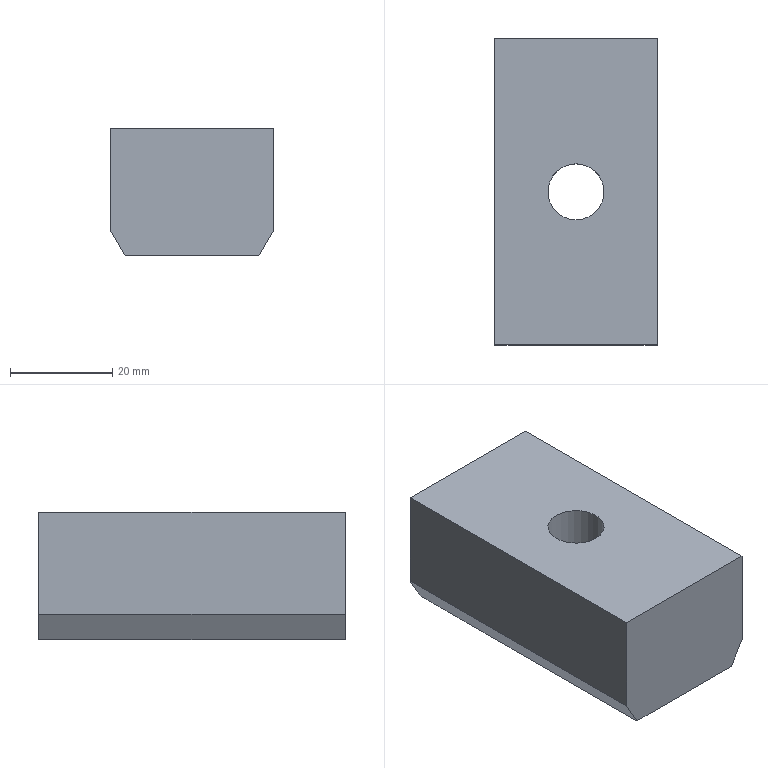Part | NX | features MAIN_BODY 2 | 1 solid | 11 faces | box 32 x 60 x 25 mm | volume 42845 mm3 | plane 9 | cylinder 2 | commonest cylinder face diameters 11 x1 18 x1
STEP:
#1=CARTESIAN_POINT('',(-127.887,-123.5,-120.));
#2=VERTEX_POINT('',#1);
#3=CARTESIAN_POINT('',(-154.113,-123.5,-120.));
#4=VERTEX_POINT('',#3);
#5=CARTESIAN_POINT('',(-125.,-123.5,-120.));
#6=DIRECTION('',(-1.,0.,0.));
#7=VECTOR('',#6,1000.);
#8=LINE('',#5,#7);
#9=EDGE_CURVE('',#2,#4,#8,.T.);
#10=ORIENTED_EDGE('',*,*,#9,.F.);
#11=CARTESIAN_POINT('',(-125.,-123.5,-115.));
#12=VERTEX_POINT('',#11);
#13=CARTESIAN_POINT('',(-127.165,-123.5,-118.75));
#14=DIRECTION('',(-0.5,0.,-0.866));
#15=VECTOR('',#14,1000.);
#16=LINE('',#13,#15);
#17=EDGE_CURVE('',#12,#2,#16,.T.);
#18=ORIENTED_EDGE('',*,*,#17,.F.);
#19=CARTESIAN_POINT('',(-125.,-123.5,-95.));
#20=VERTEX_POINT('',#19);
#21=CARTESIAN_POINT('',(-125.,-123.5,-120.));
#22=DIRECTION('',(0.,0.,1.));
#23=VECTOR('',#22,1000.);
#24=LINE('',#21,#23);
#25=EDGE_CURVE('',#12,#20,#24,.T.);
#26=ORIENTED_EDGE('',*,*,#25,.T.);
#27=CARTESIAN_POINT('',(-157.,-123.5,-95.));
#28=VERTEX_POINT('',#27);
#29=CARTESIAN_POINT('',(-125.,-123.5,-95.));
#30=DIRECTION('',(-1.,0.,0.));
#31=VECTOR('',#30,1000.);
#32=LINE('',#29,#31);
#33=EDGE_CURVE('',#20,#28,#32,.T.);
#34=ORIENTED_EDGE('',*,*,#33,.T.);
#35=CARTESIAN_POINT('',(-157.,-123.5,-115.));
#36=VERTEX_POINT('',#35);
#37=CARTESIAN_POINT('',(-157.,-123.5,-120.));
#38=DIRECTION('',(0.,0.,1.));
#39=VECTOR('',#38,1000.);
#40=LINE('',#37,#39);
#41=EDGE_CURVE('',#36,#28,#40,.T.);
#42=ORIENTED_EDGE('',*,*,#41,.F.);
#43=CARTESIAN_POINT('',(-146.835,-123.5,-132.606));
#44=DIRECTION('',(-0.5,0.,0.866));
#45=VECTOR('',#44,1000.);
#46=LINE('',#43,#45);
#47=EDGE_CURVE('',#4,#36,#46,.T.);
#48=ORIENTED_EDGE('',*,*,#47,.F.);
#49=EDGE_LOOP('',(#10,#18,#26,#34,#42,#48));
#50=FACE_BOUND('',#49,.T.);
#51=CARTESIAN_POINT('',(-125.,-123.5,-120.));
#52=DIRECTION('',(0.,-1.,0.));
#53=DIRECTION('',(1.,0.,0.));
#54=AXIS2_PLACEMENT_3D('',#51,#52,#53);
#55=PLANE('',#54);
#56=ADVANCED_FACE('',(#50),#55,.T.);
#57=ORIENTED_EDGE('',*,*,#41,.T.);
#58=CARTESIAN_POINT('',(-157.,-63.5,-95.));
#59=VERTEX_POINT('',#58);
#60=CARTESIAN_POINT('',(-157.,-123.5,-95.));
#61=DIRECTION('',(0.,1.,0.));
#62=VECTOR('',#61,1000.);
#63=LINE('',#60,#62);
#64=EDGE_CURVE('',#28,#59,#63,.T.);
#65=ORIENTED_EDGE('',*,*,#64,.T.);
#66=CARTESIAN_POINT('',(-157.,-63.5,-115.));
#67=VERTEX_POINT('',#66);
#68=CARTESIAN_POINT('',(-157.,-63.5,-120.));
#69=DIRECTION('',(0.,0.,1.));
#70=VECTOR('',#69,1000.);
#71=LINE('',#68,#70);
#72=EDGE_CURVE('',#67,#59,#71,.T.);
#73=ORIENTED_EDGE('',*,*,#72,.F.);
#74=CARTESIAN_POINT('',(-157.,-63.5,-115.));
#75=DIRECTION('',(0.,1.,0.));
#76=VECTOR('',#75,1000.);
#77=LINE('',#74,#76);
#78=EDGE_CURVE('',#36,#67,#77,.T.);
#79=ORIENTED_EDGE('',*,*,#78,.F.);
#80=EDGE_LOOP('',(#57,#65,#73,#79));
#81=FACE_BOUND('',#80,.T.);
#82=CARTESIAN_POINT('',(-157.,-123.5,-120.));
#83=DIRECTION('',(-1.,0.,0.));
#84=DIRECTION('',(0.,-1.,0.));
#85=AXIS2_PLACEMENT_3D('',#82,#83,#84);
#86=PLANE('',#85);
#87=ADVANCED_FACE('',(#81),#86,.T.);
#88=ORIENTED_EDGE('',*,*,#72,.T.);
#89=CARTESIAN_POINT('',(-125.,-63.5,-95.));
#90=VERTEX_POINT('',#89);
#91=CARTESIAN_POINT('',(-157.,-63.5,-95.));
#92=DIRECTION('',(1.,0.,0.));
#93=VECTOR('',#92,1000.);
#94=LINE('',#91,#93);
#95=EDGE_CURVE('',#59,#90,#94,.T.);
#96=ORIENTED_EDGE('',*,*,#95,.T.);
#97=CARTESIAN_POINT('',(-125.,-63.5,-115.));
#98=VERTEX_POINT('',#97);
#99=CARTESIAN_POINT('',(-125.,-63.5,-120.));
#100=DIRECTION('',(0.,0.,1.));
#101=VECTOR('',#100,1000.);
#102=LINE('',#99,#101);
#103=EDGE_CURVE('',#98,#90,#102,.T.);
#104=ORIENTED_EDGE('',*,*,#103,.F.);
#105=CARTESIAN_POINT('',(-127.887,-63.5,-120.));
#106=VERTEX_POINT('',#105);
#107=CARTESIAN_POINT('',(-135.165,-63.5,-132.606));
#108=DIRECTION('',(0.5,0.,0.866));
#109=VECTOR('',#108,1000.);
#110=LINE('',#107,#109);
#111=EDGE_CURVE('',#106,#98,#110,.T.);
#112=ORIENTED_EDGE('',*,*,#111,.F.);
#113=CARTESIAN_POINT('',(-154.113,-63.5,-120.));
#114=VERTEX_POINT('',#113);
#115=CARTESIAN_POINT('',(-157.,-63.5,-120.));
#116=DIRECTION('',(1.,0.,0.));
#117=VECTOR('',#116,1000.);
#118=LINE('',#115,#117);
#119=EDGE_CURVE('',#114,#106,#118,.T.);
#120=ORIENTED_EDGE('',*,*,#119,.F.);
#121=CARTESIAN_POINT('',(-154.835,-63.5,-118.75));
#122=DIRECTION('',(0.5,0.,-0.866));
#123=VECTOR('',#122,1000.);
#124=LINE('',#121,#123);
#125=EDGE_CURVE('',#67,#114,#124,.T.);
#126=ORIENTED_EDGE('',*,*,#125,.F.);
#127=EDGE_LOOP('',(#88,#96,#104,#112,#120,#126));
#128=FACE_BOUND('',#127,.T.);
#129=CARTESIAN_POINT('',(-157.,-63.5,-120.));
#130=DIRECTION('',(0.,1.,0.));
#131=DIRECTION('',(-1.,0.,0.));
#132=AXIS2_PLACEMENT_3D('',#129,#130,#131);
#133=PLANE('',#132);
#134=ADVANCED_FACE('',(#128),#133,.T.);
#135=ORIENTED_EDGE('',*,*,#103,.T.);
#136=CARTESIAN_POINT('',(-125.,-63.5,-95.));
#137=DIRECTION('',(0.,-1.,0.));
#138=VECTOR('',#137,1000.);
#139=LINE('',#136,#138);
#140=EDGE_CURVE('',#90,#20,#139,.T.);
#141=ORIENTED_EDGE('',*,*,#140,.T.);
#142=ORIENTED_EDGE('',*,*,#25,.F.);
#143=CARTESIAN_POINT('',(-125.,-123.5,-115.));
#144=DIRECTION('',(0.,-1.,0.));
#145=VECTOR('',#144,1000.);
#146=LINE('',#143,#145);
#147=EDGE_CURVE('',#98,#12,#146,.T.);
#148=ORIENTED_EDGE('',*,*,#147,.F.);
#149=EDGE_LOOP('',(#135,#141,#142,#148));
#150=FACE_BOUND('',#149,.T.);
#151=CARTESIAN_POINT('',(-125.,-63.5,-120.));
#152=DIRECTION('',(1.,0.,0.));
#153=DIRECTION('',(0.,0.,-1.));
#154=AXIS2_PLACEMENT_3D('',#151,#152,#153);
#155=PLANE('',#154);
#156=ADVANCED_FACE('',(#150),#155,.T.);
#157=CARTESIAN_POINT('',(-141.,-84.5,-120.));
#158=VERTEX_POINT('',#157);
#159=CARTESIAN_POINT('',(-141.,-93.5,-120.));
#160=DIRECTION('',(0.,0.,-1.));
#161=DIRECTION('',(0.,1.,0.));
#162=AXIS2_PLACEMENT_3D('',#159,#160,#161);
#163=CIRCLE('',#162,9.);
#164=EDGE_CURVE('',#158,#158,#163,.T.);
#165=ORIENTED_EDGE('',*,*,#164,.F.);
#166=EDGE_LOOP('',(#165));
#167=FACE_BOUND('',#166,.T.);
#168=ORIENTED_EDGE('',*,*,#119,.T.);
#169=CARTESIAN_POINT('',(-127.887,-63.5,-120.));
#170=DIRECTION('',(0.,1.,0.));
#171=VECTOR('',#170,1000.);
#172=LINE('',#169,#171);
#173=EDGE_CURVE('',#2,#106,#172,.T.);
#174=ORIENTED_EDGE('',*,*,#173,.F.);
#175=ORIENTED_EDGE('',*,*,#9,.T.);
#176=CARTESIAN_POINT('',(-154.113,-123.5,-120.));
#177=DIRECTION('',(0.,-1.,0.));
#178=VECTOR('',#177,1000.);
#179=LINE('',#176,#178);
#180=EDGE_CURVE('',#114,#4,#179,.T.);
#181=ORIENTED_EDGE('',*,*,#180,.F.);
#182=EDGE_LOOP('',(#168,#174,#175,#181));
#183=FACE_BOUND('',#182,.T.);
#184=CARTESIAN_POINT('',(-157.,-123.5,-120.));
#185=DIRECTION('',(0.,0.,1.));
#186=DIRECTION('',(0.,1.,0.));
#187=AXIS2_PLACEMENT_3D('',#184,#185,#186);
#188=PLANE('',#187);
#189=ADVANCED_FACE('',(#167,#183),#188,.F.);
#190=CARTESIAN_POINT('',(-141.,-88.,-95.));
#191=VERTEX_POINT('',#190);
#192=CARTESIAN_POINT('',(-141.,-93.5,-95.));
#193=DIRECTION('',(0.,0.,-1.));
#194=DIRECTION('',(0.,1.,0.));
#195=AXIS2_PLACEMENT_3D('',#192,#193,#194);
#196=CIRCLE('',#195,5.5);
#197=EDGE_CURVE('',#191,#191,#196,.T.);
#198=ORIENTED_EDGE('',*,*,#197,.T.);
#199=EDGE_LOOP('',(#198));
#200=FACE_BOUND('',#199,.T.);
#201=ORIENTED_EDGE('',*,*,#33,.F.);
#202=ORIENTED_EDGE('',*,*,#140,.F.);
#203=ORIENTED_EDGE('',*,*,#95,.F.);
#204=ORIENTED_EDGE('',*,*,#64,.F.);
#205=EDGE_LOOP('',(#201,#202,#203,#204));
#206=FACE_BOUND('',#205,.T.);
#207=CARTESIAN_POINT('',(-157.,-123.5,-95.));
#208=DIRECTION('',(0.,0.,1.));
#209=DIRECTION('',(0.,1.,0.));
#210=AXIS2_PLACEMENT_3D('',#207,#208,#209);
#211=PLANE('',#210);
#212=ADVANCED_FACE('',(#200,#206),#211,.T.);
#213=ORIENTED_EDGE('',*,*,#47,.T.);
#214=ORIENTED_EDGE('',*,*,#78,.T.);
#215=ORIENTED_EDGE('',*,*,#125,.T.);
#216=ORIENTED_EDGE('',*,*,#180,.T.);
#217=EDGE_LOOP('',(#213,#214,#215,#216));
#218=FACE_BOUND('',#217,.T.);
#219=CARTESIAN_POINT('',(-157.,-123.5,-115.));
#220=DIRECTION('',(-0.866,0.,-0.5));
#221=DIRECTION('',(-0.5,0.,0.866));
#222=AXIS2_PLACEMENT_3D('',#219,#220,#221);
#223=PLANE('',#222);
#224=ADVANCED_FACE('',(#218),#223,.T.);
#225=ORIENTED_EDGE('',*,*,#111,.T.);
#226=ORIENTED_EDGE('',*,*,#147,.T.);
#227=ORIENTED_EDGE('',*,*,#17,.T.);
#228=ORIENTED_EDGE('',*,*,#173,.T.);
#229=EDGE_LOOP('',(#225,#226,#227,#228));
#230=FACE_BOUND('',#229,.T.);
#231=CARTESIAN_POINT('',(-125.,-63.5,-115.));
#232=DIRECTION('',(0.866,0.,-0.5));
#233=DIRECTION('',(-0.5,0.,-0.866));
#234=AXIS2_PLACEMENT_3D('',#231,#232,#233);
#235=PLANE('',#234);
#236=ADVANCED_FACE('',(#230),#235,.T.);
#237=ORIENTED_EDGE('',*,*,#197,.F.);
#238=EDGE_LOOP('',(#237));
#239=FACE_BOUND('',#238,.T.);
#240=CARTESIAN_POINT('',(-141.,-88.,-108.));
#241=VERTEX_POINT('',#240);
#242=CARTESIAN_POINT('',(-141.,-93.5,-108.));
#243=DIRECTION('',(0.,0.,-1.));
#244=DIRECTION('',(0.,1.,0.));
#245=AXIS2_PLACEMENT_3D('',#242,#243,#244);
#246=CIRCLE('',#245,5.5);
#247=EDGE_CURVE('',#241,#241,#246,.T.);
#248=ORIENTED_EDGE('',*,*,#247,.T.);
#249=EDGE_LOOP('',(#248));
#250=FACE_BOUND('',#249,.T.);
#251=CARTESIAN_POINT('',(-141.,-93.5,-70.));
#252=DIRECTION('',(0.,0.,1.));
#253=DIRECTION('',(0.,1.,0.));
#254=AXIS2_PLACEMENT_3D('',#251,#252,#253);
#255=CYLINDRICAL_SURFACE('',#254,5.5);
#256=ADVANCED_FACE('',(#239,#250),#255,.F.);
#257=ORIENTED_EDGE('',*,*,#247,.F.);
#258=EDGE_LOOP('',(#257));
#259=FACE_BOUND('',#258,.T.);
#260=CARTESIAN_POINT('',(-141.,-84.5,-108.));
#261=VERTEX_POINT('',#260);
#262=CARTESIAN_POINT('',(-141.,-93.5,-108.));
#263=DIRECTION('',(0.,0.,-1.));
#264=DIRECTION('',(0.,1.,0.));
#265=AXIS2_PLACEMENT_3D('',#262,#263,#264);
#266=CIRCLE('',#265,9.);
#267=EDGE_CURVE('',#261,#261,#266,.T.);
#268=ORIENTED_EDGE('',*,*,#267,.T.);
#269=EDGE_LOOP('',(#268));
#270=FACE_BOUND('',#269,.T.);
#271=CARTESIAN_POINT('',(-141.,-93.5,-108.));
#272=DIRECTION('',(0.,0.,1.));
#273=DIRECTION('',(0.,1.,0.));
#274=AXIS2_PLACEMENT_3D('',#271,#272,#273);
#275=PLANE('',#274);
#276=ADVANCED_FACE('',(#259,#270),#275,.F.);
#277=ORIENTED_EDGE('',*,*,#267,.F.);
#278=EDGE_LOOP('',(#277));
#279=FACE_BOUND('',#278,.T.);
#280=ORIENTED_EDGE('',*,*,#164,.T.);
#281=EDGE_LOOP('',(#280));
#282=FACE_BOUND('',#281,.T.);
#283=CARTESIAN_POINT('',(-141.,-93.5,-120.));
#284=DIRECTION('',(0.,0.,1.));
#285=DIRECTION('',(0.,1.,0.));
#286=AXIS2_PLACEMENT_3D('',#283,#284,#285);
#287=CYLINDRICAL_SURFACE('',#286,9.);
#288=ADVANCED_FACE('',(#279,#282),#287,.F.);
#289=CLOSED_SHELL('',(#56,#87,#134,#156,#189,#212,#224,#236,#256,#276,#288));
#290=MANIFOLD_SOLID_BREP('',#289);
#291=(LENGTH_UNIT()NAMED_UNIT(*)SI_UNIT(.MILLI.,.METRE.));
#292=UNCERTAINTY_MEASURE_WITH_UNIT(LENGTH_MEASURE(0.00001),#291,'','');
#293=(NAMED_UNIT(*)PLANE_ANGLE_UNIT()SI_UNIT($,.RADIAN.));
#294=(NAMED_UNIT(*)SI_UNIT($,.STERADIAN.)SOLID_ANGLE_UNIT());
#295=(GEOMETRIC_REPRESENTATION_CONTEXT(3)GLOBAL_UNCERTAINTY_ASSIGNED_CONTEXT((#292))GLOBAL_UNIT_ASSIGNED_CONTEXT((#291,#293,#294))REPRESENTATION_CONTEXT('',''));
#296=ADVANCED_BREP_SHAPE_REPRESENTATION('',(#290),#295);